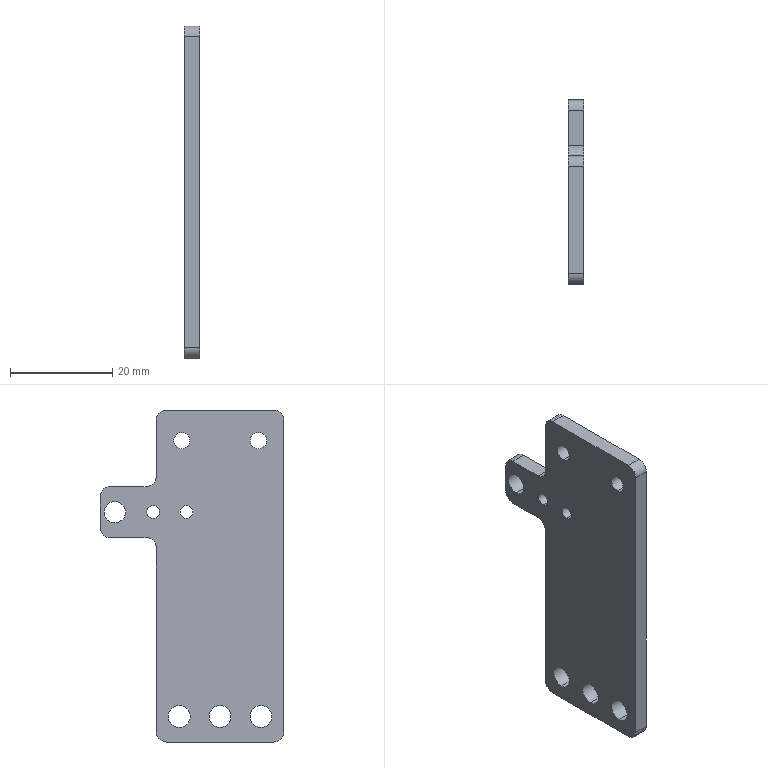Part | SolidWorks | features Fillet 2, HoleWzd 2, ICE 2, Extrusion 1 | 1 solid | 34 faces | box 3 x 36 x 65 mm | volume 4945 mm3 | cylinder 24 | plane 10 | commonest cylinder face diameters 4 x8 4.3 x6 2.5 x4 3.2 x4 4.2 x2
STEP:
#1=CARTESIAN_POINT('',(3.,6.6,13.75));
#2=VERTEX_POINT('',#1);
#3=CARTESIAN_POINT('',(3.,6.6,11.25));
#4=VERTEX_POINT('',#3);
#5=CARTESIAN_POINT('',(3.,6.6,12.5));
#6=DIRECTION('',(1.,0.,0.));
#7=DIRECTION('',(0.,0.,-1.));
#8=AXIS2_PLACEMENT_3D('',#5,#6,#7);
#9=CIRCLE('',#8,1.25);
#10=EDGE_CURVE('',#2,#4,#9,.T.);
#11=ORIENTED_EDGE('',*,*,#10,.T.);
#12=CARTESIAN_POINT('',(0.,6.6,11.25));
#13=VERTEX_POINT('',#12);
#14=CARTESIAN_POINT('',(0.,6.6,11.25));
#15=DIRECTION('',(-1.,0.,0.));
#16=VECTOR('',#15,1000.);
#17=LINE('',#14,#16);
#18=EDGE_CURVE('',#4,#13,#17,.T.);
#19=ORIENTED_EDGE('',*,*,#18,.T.);
#20=CARTESIAN_POINT('',(0.,6.6,13.75));
#21=VERTEX_POINT('',#20);
#22=CARTESIAN_POINT('',(0.,6.6,12.5));
#23=DIRECTION('',(-1.,0.,0.));
#24=DIRECTION('',(0.,0.,1.));
#25=AXIS2_PLACEMENT_3D('',#22,#23,#24);
#26=CIRCLE('',#25,1.25);
#27=EDGE_CURVE('',#13,#21,#26,.T.);
#28=ORIENTED_EDGE('',*,*,#27,.T.);
#29=CARTESIAN_POINT('',(0.,6.6,13.75));
#30=DIRECTION('',(-1.,0.,0.));
#31=VECTOR('',#30,1000.);
#32=LINE('',#29,#31);
#33=EDGE_CURVE('',#2,#21,#32,.T.);
#34=ORIENTED_EDGE('',*,*,#33,.F.);
#35=EDGE_LOOP('',(#11,#19,#28,#34));
#36=FACE_OUTER_BOUND('',#35,.T.);
#37=CARTESIAN_POINT('',(0.,6.6,12.5));
#38=DIRECTION('',(-1.,0.,0.));
#39=DIRECTION('',(0.,0.,1.));
#40=AXIS2_PLACEMENT_3D('',#37,#38,#39);
#41=CYLINDRICAL_SURFACE('',#40,1.25);
#42=ADVANCED_FACE('',(#36),#41,.F.);
#43=CARTESIAN_POINT('',(3.,13.1,13.75));
#44=VERTEX_POINT('',#43);
#45=CARTESIAN_POINT('',(3.,13.1,11.25));
#46=VERTEX_POINT('',#45);
#47=CARTESIAN_POINT('',(3.,13.1,12.5));
#48=DIRECTION('',(1.,0.,0.));
#49=DIRECTION('',(0.,0.,-1.));
#50=AXIS2_PLACEMENT_3D('',#47,#48,#49);
#51=CIRCLE('',#50,1.25);
#52=EDGE_CURVE('',#44,#46,#51,.T.);
#53=ORIENTED_EDGE('',*,*,#52,.T.);
#54=CARTESIAN_POINT('',(0.,13.1,11.25));
#55=VERTEX_POINT('',#54);
#56=CARTESIAN_POINT('',(0.,13.1,11.25));
#57=DIRECTION('',(-1.,0.,0.));
#58=VECTOR('',#57,1000.);
#59=LINE('',#56,#58);
#60=EDGE_CURVE('',#46,#55,#59,.T.);
#61=ORIENTED_EDGE('',*,*,#60,.T.);
#62=CARTESIAN_POINT('',(0.,13.1,13.75));
#63=VERTEX_POINT('',#62);
#64=CARTESIAN_POINT('',(0.,13.1,12.5));
#65=DIRECTION('',(-1.,0.,0.));
#66=DIRECTION('',(0.,0.,1.));
#67=AXIS2_PLACEMENT_3D('',#64,#65,#66);
#68=CIRCLE('',#67,1.25);
#69=EDGE_CURVE('',#55,#63,#68,.T.);
#70=ORIENTED_EDGE('',*,*,#69,.T.);
#71=CARTESIAN_POINT('',(0.,13.1,13.75));
#72=DIRECTION('',(-1.,0.,0.));
#73=VECTOR('',#72,1000.);
#74=LINE('',#71,#73);
#75=EDGE_CURVE('',#44,#63,#74,.T.);
#76=ORIENTED_EDGE('',*,*,#75,.F.);
#77=EDGE_LOOP('',(#53,#61,#70,#76));
#78=FACE_OUTER_BOUND('',#77,.T.);
#79=CARTESIAN_POINT('',(0.,13.1,12.5));
#80=DIRECTION('',(-1.,0.,0.));
#81=DIRECTION('',(0.,0.,1.));
#82=AXIS2_PLACEMENT_3D('',#79,#80,#81);
#83=CYLINDRICAL_SURFACE('',#82,1.25);
#84=ADVANCED_FACE('',(#78),#83,.F.);
#85=CARTESIAN_POINT('',(3.,20.6,14.6));
#86=VERTEX_POINT('',#85);
#87=CARTESIAN_POINT('',(3.,20.6,10.4));
#88=VERTEX_POINT('',#87);
#89=CARTESIAN_POINT('',(3.,20.6,12.5));
#90=DIRECTION('',(1.,0.,0.));
#91=DIRECTION('',(0.,0.,-1.));
#92=AXIS2_PLACEMENT_3D('',#89,#90,#91);
#93=CIRCLE('',#92,2.1);
#94=EDGE_CURVE('',#86,#88,#93,.T.);
#95=ORIENTED_EDGE('',*,*,#94,.T.);
#96=CARTESIAN_POINT('',(0.,20.6,10.4));
#97=VERTEX_POINT('',#96);
#98=CARTESIAN_POINT('',(10.,20.6,10.4));
#99=DIRECTION('',(-1.,0.,0.));
#100=VECTOR('',#99,1000.);
#101=LINE('',#98,#100);
#102=EDGE_CURVE('',#88,#97,#101,.T.);
#103=ORIENTED_EDGE('',*,*,#102,.T.);
#104=CARTESIAN_POINT('',(0.,20.6,14.6));
#105=VERTEX_POINT('',#104);
#106=CARTESIAN_POINT('',(0.,20.6,12.5));
#107=DIRECTION('',(-1.,0.,0.));
#108=DIRECTION('',(0.,0.,1.));
#109=AXIS2_PLACEMENT_3D('',#106,#107,#108);
#110=CIRCLE('',#109,2.1);
#111=EDGE_CURVE('',#97,#105,#110,.T.);
#112=ORIENTED_EDGE('',*,*,#111,.T.);
#113=CARTESIAN_POINT('',(10.,20.6,14.6));
#114=DIRECTION('',(-1.,0.,0.));
#115=VECTOR('',#114,1000.);
#116=LINE('',#113,#115);
#117=EDGE_CURVE('',#86,#105,#116,.T.);
#118=ORIENTED_EDGE('',*,*,#117,.F.);
#119=EDGE_LOOP('',(#95,#103,#112,#118));
#120=FACE_OUTER_BOUND('',#119,.T.);
#121=CARTESIAN_POINT('',(10.,20.6,12.5));
#122=DIRECTION('',(-1.,0.,0.));
#123=DIRECTION('',(0.,0.,1.));
#124=AXIS2_PLACEMENT_3D('',#121,#122,#123);
#125=CYLINDRICAL_SURFACE('',#124,2.1);
#126=ADVANCED_FACE('',(#120),#125,.F.);
#127=CARTESIAN_POINT('',(3.,8.,-25.35));
#128=VERTEX_POINT('',#127);
#129=CARTESIAN_POINT('',(3.,8.,-29.65));
#130=VERTEX_POINT('',#129);
#131=CARTESIAN_POINT('',(3.,8.,-27.5));
#132=DIRECTION('',(1.,0.,0.));
#133=DIRECTION('',(0.,0.,-1.));
#134=AXIS2_PLACEMENT_3D('',#131,#132,#133);
#135=CIRCLE('',#134,2.15);
#136=EDGE_CURVE('',#128,#130,#135,.T.);
#137=ORIENTED_EDGE('',*,*,#136,.T.);
#138=CARTESIAN_POINT('',(0.,8.,-29.65));
#139=VERTEX_POINT('',#138);
#140=CARTESIAN_POINT('',(0.,8.,-29.65));
#141=DIRECTION('',(-1.,0.,0.));
#142=VECTOR('',#141,1000.);
#143=LINE('',#140,#142);
#144=EDGE_CURVE('',#130,#139,#143,.T.);
#145=ORIENTED_EDGE('',*,*,#144,.T.);
#146=CARTESIAN_POINT('',(0.,8.,-25.35));
#147=VERTEX_POINT('',#146);
#148=CARTESIAN_POINT('',(0.,8.,-27.5));
#149=DIRECTION('',(-1.,0.,0.));
#150=DIRECTION('',(0.,0.,1.));
#151=AXIS2_PLACEMENT_3D('',#148,#149,#150);
#152=CIRCLE('',#151,2.15);
#153=EDGE_CURVE('',#139,#147,#152,.T.);
#154=ORIENTED_EDGE('',*,*,#153,.T.);
#155=CARTESIAN_POINT('',(0.,8.,-25.35));
#156=DIRECTION('',(-1.,0.,0.));
#157=VECTOR('',#156,1000.);
#158=LINE('',#155,#157);
#159=EDGE_CURVE('',#128,#147,#158,.T.);
#160=ORIENTED_EDGE('',*,*,#159,.F.);
#161=EDGE_LOOP('',(#137,#145,#154,#160));
#162=FACE_OUTER_BOUND('',#161,.T.);
#163=CARTESIAN_POINT('',(0.,8.,-27.5));
#164=DIRECTION('',(-1.,0.,0.));
#165=DIRECTION('',(0.,0.,1.));
#166=AXIS2_PLACEMENT_3D('',#163,#164,#165);
#167=CYLINDRICAL_SURFACE('',#166,2.15);
#168=ADVANCED_FACE('',(#162),#167,.F.);
#169=CARTESIAN_POINT('',(3.,-8.,-25.35));
#170=VERTEX_POINT('',#169);
#171=CARTESIAN_POINT('',(3.,-8.,-29.65));
#172=VERTEX_POINT('',#171);
#173=CARTESIAN_POINT('',(3.,-8.,-27.5));
#174=DIRECTION('',(1.,0.,0.));
#175=DIRECTION('',(0.,0.,-1.));
#176=AXIS2_PLACEMENT_3D('',#173,#174,#175);
#177=CIRCLE('',#176,2.15);
#178=EDGE_CURVE('',#170,#172,#177,.T.);
#179=ORIENTED_EDGE('',*,*,#178,.T.);
#180=CARTESIAN_POINT('',(0.,-8.,-29.65));
#181=VERTEX_POINT('',#180);
#182=CARTESIAN_POINT('',(0.,-8.,-29.65));
#183=DIRECTION('',(-1.,0.,0.));
#184=VECTOR('',#183,1000.);
#185=LINE('',#182,#184);
#186=EDGE_CURVE('',#172,#181,#185,.T.);
#187=ORIENTED_EDGE('',*,*,#186,.T.);
#188=CARTESIAN_POINT('',(0.,-8.,-25.35));
#189=VERTEX_POINT('',#188);
#190=CARTESIAN_POINT('',(0.,-8.,-27.5));
#191=DIRECTION('',(-1.,0.,0.));
#192=DIRECTION('',(0.,0.,1.));
#193=AXIS2_PLACEMENT_3D('',#190,#191,#192);
#194=CIRCLE('',#193,2.15);
#195=EDGE_CURVE('',#181,#189,#194,.T.);
#196=ORIENTED_EDGE('',*,*,#195,.T.);
#197=CARTESIAN_POINT('',(0.,-8.,-25.35));
#198=DIRECTION('',(-1.,0.,0.));
#199=VECTOR('',#198,1000.);
#200=LINE('',#197,#199);
#201=EDGE_CURVE('',#170,#189,#200,.T.);
#202=ORIENTED_EDGE('',*,*,#201,.F.);
#203=EDGE_LOOP('',(#179,#187,#196,#202));
#204=FACE_OUTER_BOUND('',#203,.T.);
#205=CARTESIAN_POINT('',(0.,-8.,-27.5));
#206=DIRECTION('',(-1.,0.,0.));
#207=DIRECTION('',(0.,0.,1.));
#208=AXIS2_PLACEMENT_3D('',#205,#206,#207);
#209=CYLINDRICAL_SURFACE('',#208,2.15);
#210=ADVANCED_FACE('',(#204),#209,.F.);
#211=CARTESIAN_POINT('',(3.,0.,-25.35));
#212=VERTEX_POINT('',#211);
#213=CARTESIAN_POINT('',(3.,0.,-29.65));
#214=VERTEX_POINT('',#213);
#215=CARTESIAN_POINT('',(3.,0.,-27.5));
#216=DIRECTION('',(1.,0.,0.));
#217=DIRECTION('',(0.,0.,-1.));
#218=AXIS2_PLACEMENT_3D('',#215,#216,#217);
#219=CIRCLE('',#218,2.15);
#220=EDGE_CURVE('',#212,#214,#219,.T.);
#221=ORIENTED_EDGE('',*,*,#220,.T.);
#222=CARTESIAN_POINT('',(0.,0.,-29.65));
#223=VERTEX_POINT('',#222);
#224=CARTESIAN_POINT('',(0.,0.,-29.65));
#225=DIRECTION('',(-1.,0.,0.));
#226=VECTOR('',#225,1000.);
#227=LINE('',#224,#226);
#228=EDGE_CURVE('',#214,#223,#227,.T.);
#229=ORIENTED_EDGE('',*,*,#228,.T.);
#230=CARTESIAN_POINT('',(0.,0.,-25.35));
#231=VERTEX_POINT('',#230);
#232=CARTESIAN_POINT('',(0.,0.,-27.5));
#233=DIRECTION('',(-1.,0.,0.));
#234=DIRECTION('',(0.,0.,1.));
#235=AXIS2_PLACEMENT_3D('',#232,#233,#234);
#236=CIRCLE('',#235,2.15);
#237=EDGE_CURVE('',#223,#231,#236,.T.);
#238=ORIENTED_EDGE('',*,*,#237,.T.);
#239=CARTESIAN_POINT('',(0.,0.,-25.35));
#240=DIRECTION('',(-1.,0.,0.));
#241=VECTOR('',#240,1000.);
#242=LINE('',#239,#241);
#243=EDGE_CURVE('',#212,#231,#242,.T.);
#244=ORIENTED_EDGE('',*,*,#243,.F.);
#245=EDGE_LOOP('',(#221,#229,#238,#244));
#246=FACE_OUTER_BOUND('',#245,.T.);
#247=CARTESIAN_POINT('',(0.,0.,-27.5));
#248=DIRECTION('',(-1.,0.,0.));
#249=DIRECTION('',(0.,0.,1.));
#250=AXIS2_PLACEMENT_3D('',#247,#248,#249);
#251=CYLINDRICAL_SURFACE('',#250,2.15);
#252=ADVANCED_FACE('',(#246),#251,.F.);
#253=CARTESIAN_POINT('',(3.,-7.5,28.1));
#254=VERTEX_POINT('',#253);
#255=CARTESIAN_POINT('',(3.,-7.5,24.9));
#256=VERTEX_POINT('',#255);
#257=CARTESIAN_POINT('',(3.,-7.5,26.5));
#258=DIRECTION('',(1.,0.,0.));
#259=DIRECTION('',(0.,0.,1.));
#260=AXIS2_PLACEMENT_3D('',#257,#258,#259);
#261=CIRCLE('',#260,1.6);
#262=EDGE_CURVE('',#254,#256,#261,.T.);
#263=ORIENTED_EDGE('',*,*,#262,.T.);
#264=CARTESIAN_POINT('',(0.,-7.5,24.9));
#265=VERTEX_POINT('',#264);
#266=CARTESIAN_POINT('',(3.,-7.5,24.9));
#267=DIRECTION('',(-1.,0.,0.));
#268=VECTOR('',#267,1000.);
#269=LINE('',#266,#268);
#270=EDGE_CURVE('',#256,#265,#269,.T.);
#271=ORIENTED_EDGE('',*,*,#270,.T.);
#272=CARTESIAN_POINT('',(0.,-7.5,28.1));
#273=VERTEX_POINT('',#272);
#274=CARTESIAN_POINT('',(0.,-7.5,26.5));
#275=DIRECTION('',(1.,0.,0.));
#276=DIRECTION('',(0.,0.,1.));
#277=AXIS2_PLACEMENT_3D('',#274,#275,#276);
#278=CIRCLE('',#277,1.6);
#279=EDGE_CURVE('',#273,#265,#278,.T.);
#280=ORIENTED_EDGE('',*,*,#279,.F.);
#281=CARTESIAN_POINT('',(3.,-7.5,28.1));
#282=DIRECTION('',(-1.,0.,0.));
#283=VECTOR('',#282,1000.);
#284=LINE('',#281,#283);
#285=EDGE_CURVE('',#254,#273,#284,.T.);
#286=ORIENTED_EDGE('',*,*,#285,.F.);
#287=EDGE_LOOP('',(#263,#271,#280,#286));
#288=FACE_OUTER_BOUND('',#287,.T.);
#289=CARTESIAN_POINT('',(3.,-7.5,26.5));
#290=DIRECTION('',(-1.,0.,0.));
#291=DIRECTION('',(0.,0.,1.));
#292=AXIS2_PLACEMENT_3D('',#289,#290,#291);
#293=CYLINDRICAL_SURFACE('',#292,1.6);
#294=ADVANCED_FACE('',(#288),#293,.F.);
#295=CARTESIAN_POINT('',(3.,7.5,28.1));
#296=VERTEX_POINT('',#295);
#297=CARTESIAN_POINT('',(3.,7.5,24.9));
#298=VERTEX_POINT('',#297);
#299=CARTESIAN_POINT('',(3.,7.5,26.5));
#300=DIRECTION('',(1.,0.,0.));
#301=DIRECTION('',(0.,0.,-1.));
#302=AXIS2_PLACEMENT_3D('',#299,#300,#301);
#303=CIRCLE('',#302,1.6);
#304=EDGE_CURVE('',#296,#298,#303,.T.);
#305=ORIENTED_EDGE('',*,*,#304,.T.);
#306=CARTESIAN_POINT('',(0.,7.5,24.9));
#307=VERTEX_POINT('',#306);
#308=CARTESIAN_POINT('',(3.,7.5,24.9));
#309=DIRECTION('',(-1.,0.,0.));
#310=VECTOR('',#309,1000.);
#311=LINE('',#308,#310);
#312=EDGE_CURVE('',#298,#307,#311,.T.);
#313=ORIENTED_EDGE('',*,*,#312,.T.);
#314=CARTESIAN_POINT('',(0.,7.5,28.1));
#315=VERTEX_POINT('',#314);
#316=CARTESIAN_POINT('',(0.,7.5,26.5));
#317=DIRECTION('',(1.,0.,0.));
#318=DIRECTION('',(0.,0.,-1.));
#319=AXIS2_PLACEMENT_3D('',#316,#317,#318);
#320=CIRCLE('',#319,1.6);
#321=EDGE_CURVE('',#315,#307,#320,.T.);
#322=ORIENTED_EDGE('',*,*,#321,.F.);
#323=CARTESIAN_POINT('',(3.,7.5,28.1));
#324=DIRECTION('',(-1.,0.,0.));
#325=VECTOR('',#324,1000.);
#326=LINE('',#323,#325);
#327=EDGE_CURVE('',#296,#315,#326,.T.);
#328=ORIENTED_EDGE('',*,*,#327,.F.);
#329=EDGE_LOOP('',(#305,#313,#322,#328));
#330=FACE_OUTER_BOUND('',#329,.T.);
#331=CARTESIAN_POINT('',(3.,7.5,26.5));
#332=DIRECTION('',(-1.,0.,0.));
#333=DIRECTION('',(0.,0.,1.));
#334=AXIS2_PLACEMENT_3D('',#331,#332,#333);
#335=CYLINDRICAL_SURFACE('',#334,1.6);
#336=ADVANCED_FACE('',(#330),#335,.F.);
#337=CARTESIAN_POINT('',(0.,12.5,-30.5));
#338=VERTEX_POINT('',#337);
#339=CARTESIAN_POINT('',(0.,12.5,5.5));
#340=VERTEX_POINT('',#339);
#341=CARTESIAN_POINT('',(0.,12.5,32.5));
#342=DIRECTION('',(0.,0.,1.));
#343=VECTOR('',#342,1000.);
#344=LINE('',#341,#343);
#345=EDGE_CURVE('',#338,#340,#344,.T.);
#346=ORIENTED_EDGE('',*,*,#345,.T.);
#347=CARTESIAN_POINT('',(3.,12.5,5.5));
#348=VERTEX_POINT('',#347);
#349=CARTESIAN_POINT('',(3.,12.5,5.5));
#350=DIRECTION('',(1.,0.,0.));
#351=VECTOR('',#350,1000.);
#352=LINE('',#349,#351);
#353=EDGE_CURVE('',#340,#348,#352,.T.);
#354=ORIENTED_EDGE('',*,*,#353,.T.);
#355=CARTESIAN_POINT('',(3.,12.5,-30.5));
#356=VERTEX_POINT('',#355);
#357=CARTESIAN_POINT('',(3.,12.5,32.5));
#358=DIRECTION('',(0.,0.,1.));
#359=VECTOR('',#358,1000.);
#360=LINE('',#357,#359);
#361=EDGE_CURVE('',#356,#348,#360,.T.);
#362=ORIENTED_EDGE('',*,*,#361,.F.);
#363=CARTESIAN_POINT('',(3.,12.5,-30.5));
#364=DIRECTION('',(-1.,0.,0.));
#365=VECTOR('',#364,1000.);
#366=LINE('',#363,#365);
#367=EDGE_CURVE('',#356,#338,#366,.T.);
#368=ORIENTED_EDGE('',*,*,#367,.T.);
#369=EDGE_LOOP('',(#346,#354,#362,#368));
#370=FACE_OUTER_BOUND('',#369,.T.);
#371=CARTESIAN_POINT('',(3.,12.5,32.5));
#372=DIRECTION('',(0.,-1.,0.));
#373=DIRECTION('',(0.,0.,-1.));
#374=AXIS2_PLACEMENT_3D('',#371,#372,#373);
#375=PLANE('',#374);
#376=ADVANCED_FACE('',(#370),#375,.F.);
#377=ORIENTED_EDGE('',*,*,#10,.F.);
#378=CARTESIAN_POINT('',(3.,6.6,12.5));
#379=DIRECTION('',(1.,0.,0.));
#380=DIRECTION('',(0.,0.,-1.));
#381=AXIS2_PLACEMENT_3D('',#378,#379,#380);
#382=CIRCLE('',#381,1.25);
#383=EDGE_CURVE('',#4,#2,#382,.T.);
#384=ORIENTED_EDGE('',*,*,#383,.F.);
#385=EDGE_LOOP('',(#377,#384));
#386=FACE_BOUND('',#385,.T.);
#387=ORIENTED_EDGE('',*,*,#52,.F.);
#388=CARTESIAN_POINT('',(3.,13.1,12.5));
#389=DIRECTION('',(1.,0.,0.));
#390=DIRECTION('',(0.,0.,-1.));
#391=AXIS2_PLACEMENT_3D('',#388,#389,#390);
#392=CIRCLE('',#391,1.25);
#393=EDGE_CURVE('',#46,#44,#392,.T.);
#394=ORIENTED_EDGE('',*,*,#393,.F.);
#395=EDGE_LOOP('',(#387,#394));
#396=FACE_BOUND('',#395,.T.);
#397=ORIENTED_EDGE('',*,*,#94,.F.);
#398=CARTESIAN_POINT('',(3.,20.6,12.5));
#399=DIRECTION('',(1.,0.,0.));
#400=DIRECTION('',(0.,0.,-1.));
#401=AXIS2_PLACEMENT_3D('',#398,#399,#400);
#402=CIRCLE('',#401,2.1);
#403=EDGE_CURVE('',#88,#86,#402,.T.);
#404=ORIENTED_EDGE('',*,*,#403,.F.);
#405=EDGE_LOOP('',(#397,#404));
#406=FACE_BOUND('',#405,.T.);
#407=CARTESIAN_POINT('',(3.,23.5,9.5));
#408=VERTEX_POINT('',#407);
#409=CARTESIAN_POINT('',(3.,23.5,15.5));
#410=VERTEX_POINT('',#409);
#411=CARTESIAN_POINT('',(3.,23.5,17.5));
#412=DIRECTION('',(0.,0.,1.));
#413=VECTOR('',#412,1000.);
#414=LINE('',#411,#413);
#415=EDGE_CURVE('',#408,#410,#414,.T.);
#416=ORIENTED_EDGE('',*,*,#415,.T.);
#417=CARTESIAN_POINT('',(3.,21.5,17.5));
#418=VERTEX_POINT('',#417);
#419=CARTESIAN_POINT('',(3.,21.5,15.5));
#420=DIRECTION('',(1.,0.,0.));
#421=DIRECTION('',(0.,0.,-1.));
#422=AXIS2_PLACEMENT_3D('',#419,#420,#421);
#423=CIRCLE('',#422,2.);
#424=EDGE_CURVE('',#410,#418,#423,.T.);
#425=ORIENTED_EDGE('',*,*,#424,.T.);
#426=CARTESIAN_POINT('',(3.,14.5,17.5));
#427=VERTEX_POINT('',#426);
#428=CARTESIAN_POINT('',(3.,23.5,17.5));
#429=DIRECTION('',(0.,-1.,0.));
#430=VECTOR('',#429,1000.);
#431=LINE('',#428,#430);
#432=EDGE_CURVE('',#418,#427,#431,.T.);
#433=ORIENTED_EDGE('',*,*,#432,.T.);
#434=CARTESIAN_POINT('',(3.,12.5,19.5));
#435=VERTEX_POINT('',#434);
#436=CARTESIAN_POINT('',(3.,14.5,19.5));
#437=DIRECTION('',(-1.,0.,0.));
#438=DIRECTION('',(0.,0.,-1.));
#439=AXIS2_PLACEMENT_3D('',#436,#437,#438);
#440=CIRCLE('',#439,2.);
#441=EDGE_CURVE('',#427,#435,#440,.T.);
#442=ORIENTED_EDGE('',*,*,#441,.T.);
#443=CARTESIAN_POINT('',(3.,12.5,30.5));
#444=VERTEX_POINT('',#443);
#445=CARTESIAN_POINT('',(3.,12.5,32.5));
#446=DIRECTION('',(0.,0.,1.));
#447=VECTOR('',#446,1000.);
#448=LINE('',#445,#447);
#449=EDGE_CURVE('',#435,#444,#448,.T.);
#450=ORIENTED_EDGE('',*,*,#449,.T.);
#451=CARTESIAN_POINT('',(3.,10.5,32.5));
#452=VERTEX_POINT('',#451);
#453=CARTESIAN_POINT('',(3.,10.5,30.5));
#454=DIRECTION('',(1.,0.,0.));
#455=DIRECTION('',(0.,0.,-1.));
#456=AXIS2_PLACEMENT_3D('',#453,#454,#455);
#457=CIRCLE('',#456,2.);
#458=EDGE_CURVE('',#444,#452,#457,.T.);
#459=ORIENTED_EDGE('',*,*,#458,.T.);
#460=CARTESIAN_POINT('',(3.,-10.5,32.5));
#461=VERTEX_POINT('',#460);
#462=CARTESIAN_POINT('',(3.,12.5,32.5));
#463=DIRECTION('',(0.,-1.,0.));
#464=VECTOR('',#463,1000.);
#465=LINE('',#462,#464);
#466=EDGE_CURVE('',#452,#461,#465,.T.);
#467=ORIENTED_EDGE('',*,*,#466,.T.);
#468=CARTESIAN_POINT('',(3.,-12.5,30.5));
#469=VERTEX_POINT('',#468);
#470=CARTESIAN_POINT('',(3.,-10.5,30.5));
#471=DIRECTION('',(1.,0.,0.));
#472=DIRECTION('',(0.,0.,-1.));
#473=AXIS2_PLACEMENT_3D('',#470,#471,#472);
#474=CIRCLE('',#473,2.);
#475=EDGE_CURVE('',#461,#469,#474,.T.);
#476=ORIENTED_EDGE('',*,*,#475,.T.);
#477=CARTESIAN_POINT('',(3.,-12.5,-30.5));
#478=VERTEX_POINT('',#477);
#479=CARTESIAN_POINT('',(3.,-12.5,32.5));
#480=DIRECTION('',(0.,0.,-1.));
#481=VECTOR('',#480,1000.);
#482=LINE('',#479,#481);
#483=EDGE_CURVE('',#469,#478,#482,.T.);
#484=ORIENTED_EDGE('',*,*,#483,.T.);
#485=CARTESIAN_POINT('',(3.,-10.5,-32.5));
#486=VERTEX_POINT('',#485);
#487=CARTESIAN_POINT('',(3.,-10.5,-30.5));
#488=DIRECTION('',(1.,0.,0.));
#489=DIRECTION('',(0.,0.,-1.));
#490=AXIS2_PLACEMENT_3D('',#487,#488,#489);
#491=CIRCLE('',#490,2.);
#492=EDGE_CURVE('',#478,#486,#491,.T.);
#493=ORIENTED_EDGE('',*,*,#492,.T.);
#494=CARTESIAN_POINT('',(3.,10.5,-32.5));
#495=VERTEX_POINT('',#494);
#496=CARTESIAN_POINT('',(3.,12.5,-32.5));
#497=DIRECTION('',(0.,1.,0.));
#498=VECTOR('',#497,1000.);
#499=LINE('',#496,#498);
#500=EDGE_CURVE('',#486,#495,#499,.T.);
#501=ORIENTED_EDGE('',*,*,#500,.T.);
#502=CARTESIAN_POINT('',(3.,10.5,-30.5));
#503=DIRECTION('',(1.,0.,0.));
#504=DIRECTION('',(0.,0.,-1.));
#505=AXIS2_PLACEMENT_3D('',#502,#503,#504);
#506=CIRCLE('',#505,2.);
#507=EDGE_CURVE('',#495,#356,#506,.T.);
#508=ORIENTED_EDGE('',*,*,#507,.T.);
#509=ORIENTED_EDGE('',*,*,#361,.T.);
#510=CARTESIAN_POINT('',(3.,14.5,7.5));
#511=VERTEX_POINT('',#510);
#512=CARTESIAN_POINT('',(3.,14.5,5.5));
#513=DIRECTION('',(-1.,0.,0.));
#514=DIRECTION('',(0.,0.,-1.));
#515=AXIS2_PLACEMENT_3D('',#512,#513,#514);
#516=CIRCLE('',#515,2.);
#517=EDGE_CURVE('',#348,#511,#516,.T.);
#518=ORIENTED_EDGE('',*,*,#517,.T.);
#519=CARTESIAN_POINT('',(3.,21.5,7.5));
#520=VERTEX_POINT('',#519);
#521=CARTESIAN_POINT('',(3.,23.5,7.5));
#522=DIRECTION('',(0.,1.,0.));
#523=VECTOR('',#522,1000.);
#524=LINE('',#521,#523);
#525=EDGE_CURVE('',#511,#520,#524,.T.);
#526=ORIENTED_EDGE('',*,*,#525,.T.);
#527=CARTESIAN_POINT('',(3.,21.5,9.5));
#528=DIRECTION('',(1.,0.,0.));
#529=DIRECTION('',(0.,0.,-1.));
#530=AXIS2_PLACEMENT_3D('',#527,#528,#529);
#531=CIRCLE('',#530,2.);
#532=EDGE_CURVE('',#520,#408,#531,.T.);
#533=ORIENTED_EDGE('',*,*,#532,.T.);
#534=EDGE_LOOP('',(#416,#425,#433,#442,#450,#459,#467,#476,#484,#493,#501,#508,#509,#518,#526,#533));
#535=FACE_OUTER_BOUND('',#534,.T.);
#536=ORIENTED_EDGE('',*,*,#136,.F.);
#537=CARTESIAN_POINT('',(3.,8.,-27.5));
#538=DIRECTION('',(1.,0.,0.));
#539=DIRECTION('',(0.,0.,-1.));
#540=AXIS2_PLACEMENT_3D('',#537,#538,#539);
#541=CIRCLE('',#540,2.15);
#542=EDGE_CURVE('',#130,#128,#541,.T.);
#543=ORIENTED_EDGE('',*,*,#542,.F.);
#544=EDGE_LOOP('',(#536,#543));
#545=FACE_BOUND('',#544,.T.);
#546=ORIENTED_EDGE('',*,*,#178,.F.);
#547=CARTESIAN_POINT('',(3.,-8.,-27.5));
#548=DIRECTION('',(1.,0.,0.));
#549=DIRECTION('',(0.,0.,-1.));
#550=AXIS2_PLACEMENT_3D('',#547,#548,#549);
#551=CIRCLE('',#550,2.15);
#552=EDGE_CURVE('',#172,#170,#551,.T.);
#553=ORIENTED_EDGE('',*,*,#552,.F.);
#554=EDGE_LOOP('',(#546,#553));
#555=FACE_BOUND('',#554,.T.);
#556=ORIENTED_EDGE('',*,*,#220,.F.);
#557=CARTESIAN_POINT('',(3.,0.,-27.5));
#558=DIRECTION('',(1.,0.,0.));
#559=DIRECTION('',(0.,0.,-1.));
#560=AXIS2_PLACEMENT_3D('',#557,#558,#559);
#561=CIRCLE('',#560,2.15);
#562=EDGE_CURVE('',#214,#212,#561,.T.);
#563=ORIENTED_EDGE('',*,*,#562,.F.);
#564=EDGE_LOOP('',(#556,#563));
#565=FACE_BOUND('',#564,.T.);
#566=ORIENTED_EDGE('',*,*,#304,.F.);
#567=CARTESIAN_POINT('',(3.,7.5,26.5));
#568=DIRECTION('',(1.,0.,0.));
#569=DIRECTION('',(0.,0.,-1.));
#570=AXIS2_PLACEMENT_3D('',#567,#568,#569);
#571=CIRCLE('',#570,1.6);
#572=EDGE_CURVE('',#298,#296,#571,.T.);
#573=ORIENTED_EDGE('',*,*,#572,.F.);
#574=EDGE_LOOP('',(#566,#573));
#575=FACE_BOUND('',#574,.T.);
#576=ORIENTED_EDGE('',*,*,#262,.F.);
#577=CARTESIAN_POINT('',(3.,-7.5,26.5));
#578=DIRECTION('',(1.,0.,0.));
#579=DIRECTION('',(0.,0.,1.));
#580=AXIS2_PLACEMENT_3D('',#577,#578,#579);
#581=CIRCLE('',#580,1.6);
#582=EDGE_CURVE('',#256,#254,#581,.T.);
#583=ORIENTED_EDGE('',*,*,#582,.F.);
#584=EDGE_LOOP('',(#576,#583));
#585=FACE_BOUND('',#584,.T.);
#586=CARTESIAN_POINT('',(3.,0.,0.));
#587=DIRECTION('',(1.,0.,0.));
#588=DIRECTION('',(0.,0.,-1.));
#589=AXIS2_PLACEMENT_3D('',#586,#587,#588);
#590=PLANE('',#589);
#591=ADVANCED_FACE('',(#386,#396,#406,#535,#545,#555,#565,#575,#585),#590,.T.);
#592=CARTESIAN_POINT('',(0.,6.6,12.5));
#593=DIRECTION('',(-1.,0.,0.));
#594=DIRECTION('',(0.,0.,1.));
#595=AXIS2_PLACEMENT_3D('',#592,#593,#594);
#596=CIRCLE('',#595,1.25);
#597=EDGE_CURVE('',#21,#13,#596,.T.);
#598=ORIENTED_EDGE('',*,*,#597,.F.);
#599=ORIENTED_EDGE('',*,*,#27,.F.);
#600=EDGE_LOOP('',(#598,#599));
#601=FACE_BOUND('',#600,.T.);
#602=CARTESIAN_POINT('',(0.,13.1,12.5));
#603=DIRECTION('',(-1.,0.,0.));
#604=DIRECTION('',(0.,0.,1.));
#605=AXIS2_PLACEMENT_3D('',#602,#603,#604);
#606=CIRCLE('',#605,1.25);
#607=EDGE_CURVE('',#63,#55,#606,.T.);
#608=ORIENTED_EDGE('',*,*,#607,.F.);
#609=ORIENTED_EDGE('',*,*,#69,.F.);
#610=EDGE_LOOP('',(#608,#609));
#611=FACE_BOUND('',#610,.T.);
#612=CARTESIAN_POINT('',(0.,20.6,12.5));
#613=DIRECTION('',(-1.,0.,0.));
#614=DIRECTION('',(0.,0.,1.));
#615=AXIS2_PLACEMENT_3D('',#612,#613,#614);
#616=CIRCLE('',#615,2.1);
#617=EDGE_CURVE('',#105,#97,#616,.T.);
#618=ORIENTED_EDGE('',*,*,#617,.F.);
#619=ORIENTED_EDGE('',*,*,#111,.F.);
#620=EDGE_LOOP('',(#618,#619));
#621=FACE_BOUND('',#620,.T.);
#622=CARTESIAN_POINT('',(0.,14.5,17.5));
#623=VERTEX_POINT('',#622);
#624=CARTESIAN_POINT('',(0.,21.5,17.5));
#625=VERTEX_POINT('',#624);
#626=CARTESIAN_POINT('',(0.,23.5,17.5));
#627=DIRECTION('',(0.,1.,0.));
#628=VECTOR('',#627,1000.);
#629=LINE('',#626,#628);
#630=EDGE_CURVE('',#623,#625,#629,.T.);
#631=ORIENTED_EDGE('',*,*,#630,.T.);
#632=CARTESIAN_POINT('',(0.,23.5,15.5));
#633=VERTEX_POINT('',#632);
#634=CARTESIAN_POINT('',(0.,21.5,15.5));
#635=DIRECTION('',(-1.,0.,0.));
#636=DIRECTION('',(0.,0.,-1.));
#637=AXIS2_PLACEMENT_3D('',#634,#635,#636);
#638=CIRCLE('',#637,2.);
#639=EDGE_CURVE('',#625,#633,#638,.T.);
#640=ORIENTED_EDGE('',*,*,#639,.T.);
#641=CARTESIAN_POINT('',(0.,23.5,9.5));
#642=VERTEX_POINT('',#641);
#643=CARTESIAN_POINT('',(0.,23.5,17.5));
#644=DIRECTION('',(0.,0.,-1.));
#645=VECTOR('',#644,1000.);
#646=LINE('',#643,#645);
#647=EDGE_CURVE('',#633,#642,#646,.T.);
#648=ORIENTED_EDGE('',*,*,#647,.T.);
#649=CARTESIAN_POINT('',(0.,21.5,7.5));
#650=VERTEX_POINT('',#649);
#651=CARTESIAN_POINT('',(0.,21.5,9.5));
#652=DIRECTION('',(-1.,0.,0.));
#653=DIRECTION('',(0.,0.,-1.));
#654=AXIS2_PLACEMENT_3D('',#651,#652,#653);
#655=CIRCLE('',#654,2.);
#656=EDGE_CURVE('',#642,#650,#655,.T.);
#657=ORIENTED_EDGE('',*,*,#656,.T.);
#658=CARTESIAN_POINT('',(0.,14.5,7.5));
#659=VERTEX_POINT('',#658);
#660=CARTESIAN_POINT('',(0.,23.5,7.5));
#661=DIRECTION('',(0.,-1.,0.));
#662=VECTOR('',#661,1000.);
#663=LINE('',#660,#662);
#664=EDGE_CURVE('',#650,#659,#663,.T.);
#665=ORIENTED_EDGE('',*,*,#664,.T.);
#666=CARTESIAN_POINT('',(0.,14.5,5.5));
#667=DIRECTION('',(1.,0.,0.));
#668=DIRECTION('',(0.,0.,-1.));
#669=AXIS2_PLACEMENT_3D('',#666,#667,#668);
#670=CIRCLE('',#669,2.);
#671=EDGE_CURVE('',#659,#340,#670,.T.);
#672=ORIENTED_EDGE('',*,*,#671,.T.);
#673=ORIENTED_EDGE('',*,*,#345,.F.);
#674=CARTESIAN_POINT('',(0.,10.5,-32.5));
#675=VERTEX_POINT('',#674);
#676=CARTESIAN_POINT('',(0.,10.5,-30.5));
#677=DIRECTION('',(-1.,0.,0.));
#678=DIRECTION('',(0.,0.,-1.));
#679=AXIS2_PLACEMENT_3D('',#676,#677,#678);
#680=CIRCLE('',#679,2.);
#681=EDGE_CURVE('',#338,#675,#680,.T.);
#682=ORIENTED_EDGE('',*,*,#681,.T.);
#683=CARTESIAN_POINT('',(0.,-10.5,-32.5));
#684=VERTEX_POINT('',#683);
#685=CARTESIAN_POINT('',(0.,12.5,-32.5));
#686=DIRECTION('',(0.,1.,0.));
#687=VECTOR('',#686,1000.);
#688=LINE('',#685,#687);
#689=EDGE_CURVE('',#684,#675,#688,.T.);
#690=ORIENTED_EDGE('',*,*,#689,.F.);
#691=CARTESIAN_POINT('',(0.,-12.5,-30.5));
#692=VERTEX_POINT('',#691);
#693=CARTESIAN_POINT('',(0.,-10.5,-30.5));
#694=DIRECTION('',(-1.,0.,0.));
#695=DIRECTION('',(0.,0.,-1.));
#696=AXIS2_PLACEMENT_3D('',#693,#694,#695);
#697=CIRCLE('',#696,2.);
#698=EDGE_CURVE('',#684,#692,#697,.T.);
#699=ORIENTED_EDGE('',*,*,#698,.T.);
#700=CARTESIAN_POINT('',(0.,-12.5,30.5));
#701=VERTEX_POINT('',#700);
#702=CARTESIAN_POINT('',(0.,-12.5,32.5));
#703=DIRECTION('',(0.,0.,-1.));
#704=VECTOR('',#703,1000.);
#705=LINE('',#702,#704);
#706=EDGE_CURVE('',#701,#692,#705,.T.);
#707=ORIENTED_EDGE('',*,*,#706,.F.);
#708=CARTESIAN_POINT('',(0.,-10.5,32.5));
#709=VERTEX_POINT('',#708);
#710=CARTESIAN_POINT('',(0.,-10.5,30.5));
#711=DIRECTION('',(-1.,0.,0.));
#712=DIRECTION('',(0.,0.,-1.));
#713=AXIS2_PLACEMENT_3D('',#710,#711,#712);
#714=CIRCLE('',#713,2.);
#715=EDGE_CURVE('',#701,#709,#714,.T.);
#716=ORIENTED_EDGE('',*,*,#715,.T.);
#717=CARTESIAN_POINT('',(0.,10.5,32.5));
#718=VERTEX_POINT('',#717);
#719=CARTESIAN_POINT('',(0.,12.5,32.5));
#720=DIRECTION('',(0.,-1.,0.));
#721=VECTOR('',#720,1000.);
#722=LINE('',#719,#721);
#723=EDGE_CURVE('',#718,#709,#722,.T.);
#724=ORIENTED_EDGE('',*,*,#723,.F.);
#725=CARTESIAN_POINT('',(0.,12.5,30.5));
#726=VERTEX_POINT('',#725);
#727=CARTESIAN_POINT('',(0.,10.5,30.5));
#728=DIRECTION('',(-1.,0.,0.));
#729=DIRECTION('',(0.,0.,-1.));
#730=AXIS2_PLACEMENT_3D('',#727,#728,#729);
#731=CIRCLE('',#730,2.);
#732=EDGE_CURVE('',#718,#726,#731,.T.);
#733=ORIENTED_EDGE('',*,*,#732,.T.);
#734=CARTESIAN_POINT('',(0.,12.5,19.5));
#735=VERTEX_POINT('',#734);
#736=CARTESIAN_POINT('',(0.,12.5,32.5));
#737=DIRECTION('',(0.,0.,1.));
#738=VECTOR('',#737,1000.);
#739=LINE('',#736,#738);
#740=EDGE_CURVE('',#735,#726,#739,.T.);
#741=ORIENTED_EDGE('',*,*,#740,.F.);
#742=CARTESIAN_POINT('',(0.,14.5,19.5));
#743=DIRECTION('',(1.,0.,0.));
#744=DIRECTION('',(0.,0.,-1.));
#745=AXIS2_PLACEMENT_3D('',#742,#743,#744);
#746=CIRCLE('',#745,2.);
#747=EDGE_CURVE('',#735,#623,#746,.T.);
#748=ORIENTED_EDGE('',*,*,#747,.T.);
#749=EDGE_LOOP('',(#631,#640,#648,#657,#665,#672,#673,#682,#690,#699,#707,#716,#724,#733,#741,#748));
#750=FACE_OUTER_BOUND('',#749,.T.);
#751=CARTESIAN_POINT('',(0.,8.,-27.5));
#752=DIRECTION('',(-1.,0.,0.));
#753=DIRECTION('',(0.,0.,1.));
#754=AXIS2_PLACEMENT_3D('',#751,#752,#753);
#755=CIRCLE('',#754,2.15);
#756=EDGE_CURVE('',#147,#139,#755,.T.);
#757=ORIENTED_EDGE('',*,*,#756,.F.);
#758=ORIENTED_EDGE('',*,*,#153,.F.);
#759=EDGE_LOOP('',(#757,#758));
#760=FACE_BOUND('',#759,.T.);
#761=CARTESIAN_POINT('',(0.,-8.,-27.5));
#762=DIRECTION('',(-1.,0.,0.));
#763=DIRECTION('',(0.,0.,1.));
#764=AXIS2_PLACEMENT_3D('',#761,#762,#763);
#765=CIRCLE('',#764,2.15);
#766=EDGE_CURVE('',#189,#181,#765,.T.);
#767=ORIENTED_EDGE('',*,*,#766,.F.);
#768=ORIENTED_EDGE('',*,*,#195,.F.);
#769=EDGE_LOOP('',(#767,#768));
#770=FACE_BOUND('',#769,.T.);
#771=CARTESIAN_POINT('',(0.,0.,-27.5));
#772=DIRECTION('',(-1.,0.,0.));
#773=DIRECTION('',(0.,0.,1.));
#774=AXIS2_PLACEMENT_3D('',#771,#772,#773);
#775=CIRCLE('',#774,2.15);
#776=EDGE_CURVE('',#231,#223,#775,.T.);
#777=ORIENTED_EDGE('',*,*,#776,.F.);
#778=ORIENTED_EDGE('',*,*,#237,.F.);
#779=EDGE_LOOP('',(#777,#778));
#780=FACE_BOUND('',#779,.T.);
#781=ORIENTED_EDGE('',*,*,#321,.T.);
#782=CARTESIAN_POINT('',(0.,7.5,26.5));
#783=DIRECTION('',(1.,0.,0.));
#784=DIRECTION('',(0.,0.,-1.));
#785=AXIS2_PLACEMENT_3D('',#782,#783,#784);
#786=CIRCLE('',#785,1.6);
#787=EDGE_CURVE('',#307,#315,#786,.T.);
#788=ORIENTED_EDGE('',*,*,#787,.T.);
#789=EDGE_LOOP('',(#781,#788));
#790=FACE_BOUND('',#789,.T.);
#791=ORIENTED_EDGE('',*,*,#279,.T.);
#792=CARTESIAN_POINT('',(0.,-7.5,26.5));
#793=DIRECTION('',(1.,0.,0.));
#794=DIRECTION('',(0.,0.,1.));
#795=AXIS2_PLACEMENT_3D('',#792,#793,#794);
#796=CIRCLE('',#795,1.6);
#797=EDGE_CURVE('',#265,#273,#796,.T.);
#798=ORIENTED_EDGE('',*,*,#797,.T.);
#799=EDGE_LOOP('',(#791,#798));
#800=FACE_BOUND('',#799,.T.);
#801=CARTESIAN_POINT('',(0.,0.,0.));
#802=DIRECTION('',(1.,0.,0.));
#803=DIRECTION('',(0.,0.,-1.));
#804=AXIS2_PLACEMENT_3D('',#801,#802,#803);
#805=PLANE('',#804);
#806=ADVANCED_FACE('',(#601,#611,#621,#750,#760,#770,#780,#790,#800),#805,.F.);
#807=ORIENTED_EDGE('',*,*,#500,.F.);
#808=CARTESIAN_POINT('',(3.,-10.5,-32.5));
#809=DIRECTION('',(-1.,0.,0.));
#810=VECTOR('',#809,1000.);
#811=LINE('',#808,#810);
#812=EDGE_CURVE('',#486,#684,#811,.T.);
#813=ORIENTED_EDGE('',*,*,#812,.T.);
#814=ORIENTED_EDGE('',*,*,#689,.T.);
#815=CARTESIAN_POINT('',(3.,10.5,-32.5));
#816=DIRECTION('',(1.,0.,0.));
#817=VECTOR('',#816,1000.);
#818=LINE('',#815,#817);
#819=EDGE_CURVE('',#675,#495,#818,.T.);
#820=ORIENTED_EDGE('',*,*,#819,.T.);
#821=EDGE_LOOP('',(#807,#813,#814,#820));
#822=FACE_OUTER_BOUND('',#821,.T.);
#823=CARTESIAN_POINT('',(3.,12.5,-32.5));
#824=DIRECTION('',(0.,0.,1.));
#825=DIRECTION('',(1.,0.,0.));
#826=AXIS2_PLACEMENT_3D('',#823,#824,#825);
#827=PLANE('',#826);
#828=ADVANCED_FACE('',(#822),#827,.F.);
#829=ORIENTED_EDGE('',*,*,#449,.F.);
#830=CARTESIAN_POINT('',(3.,12.5,19.5));
#831=DIRECTION('',(-1.,0.,0.));
#832=VECTOR('',#831,1000.);
#833=LINE('',#830,#832);
#834=EDGE_CURVE('',#435,#735,#833,.T.);
#835=ORIENTED_EDGE('',*,*,#834,.T.);
#836=ORIENTED_EDGE('',*,*,#740,.T.);
#837=CARTESIAN_POINT('',(3.,12.5,30.5));
#838=DIRECTION('',(1.,0.,0.));
#839=VECTOR('',#838,1000.);
#840=LINE('',#837,#839);
#841=EDGE_CURVE('',#726,#444,#840,.T.);
#842=ORIENTED_EDGE('',*,*,#841,.T.);
#843=EDGE_LOOP('',(#829,#835,#836,#842));
#844=FACE_OUTER_BOUND('',#843,.T.);
#845=CARTESIAN_POINT('',(3.,12.5,32.5));
#846=DIRECTION('',(0.,-1.,0.));
#847=DIRECTION('',(0.,0.,-1.));
#848=AXIS2_PLACEMENT_3D('',#845,#846,#847);
#849=PLANE('',#848);
#850=ADVANCED_FACE('',(#844),#849,.F.);
#851=ORIENTED_EDGE('',*,*,#723,.T.);
#852=CARTESIAN_POINT('',(3.,-10.5,32.5));
#853=DIRECTION('',(1.,0.,0.));
#854=VECTOR('',#853,1000.);
#855=LINE('',#852,#854);
#856=EDGE_CURVE('',#709,#461,#855,.T.);
#857=ORIENTED_EDGE('',*,*,#856,.T.);
#858=ORIENTED_EDGE('',*,*,#466,.F.);
#859=CARTESIAN_POINT('',(3.,10.5,32.5));
#860=DIRECTION('',(-1.,0.,0.));
#861=VECTOR('',#860,1000.);
#862=LINE('',#859,#861);
#863=EDGE_CURVE('',#452,#718,#862,.T.);
#864=ORIENTED_EDGE('',*,*,#863,.T.);
#865=EDGE_LOOP('',(#851,#857,#858,#864));
#866=FACE_OUTER_BOUND('',#865,.T.);
#867=CARTESIAN_POINT('',(3.,12.5,32.5));
#868=DIRECTION('',(0.,0.,-1.));
#869=DIRECTION('',(-1.,0.,0.));
#870=AXIS2_PLACEMENT_3D('',#867,#868,#869);
#871=PLANE('',#870);
#872=ADVANCED_FACE('',(#866),#871,.F.);
#873=ORIENTED_EDGE('',*,*,#706,.T.);
#874=CARTESIAN_POINT('',(3.,-12.5,-30.5));
#875=DIRECTION('',(1.,0.,0.));
#876=VECTOR('',#875,1000.);
#877=LINE('',#874,#876);
#878=EDGE_CURVE('',#692,#478,#877,.T.);
#879=ORIENTED_EDGE('',*,*,#878,.T.);
#880=ORIENTED_EDGE('',*,*,#483,.F.);
#881=CARTESIAN_POINT('',(3.,-12.5,30.5));
#882=DIRECTION('',(-1.,0.,0.));
#883=VECTOR('',#882,1000.);
#884=LINE('',#881,#883);
#885=EDGE_CURVE('',#469,#701,#884,.T.);
#886=ORIENTED_EDGE('',*,*,#885,.T.);
#887=EDGE_LOOP('',(#873,#879,#880,#886));
#888=FACE_OUTER_BOUND('',#887,.T.);
#889=CARTESIAN_POINT('',(3.,-12.5,32.5));
#890=DIRECTION('',(0.,1.,0.));
#891=DIRECTION('',(0.,0.,1.));
#892=AXIS2_PLACEMENT_3D('',#889,#890,#891);
#893=PLANE('',#892);
#894=ADVANCED_FACE('',(#888),#893,.F.);
#895=ORIENTED_EDGE('',*,*,#312,.F.);
#896=ORIENTED_EDGE('',*,*,#572,.T.);
#897=ORIENTED_EDGE('',*,*,#327,.T.);
#898=ORIENTED_EDGE('',*,*,#787,.F.);
#899=EDGE_LOOP('',(#895,#896,#897,#898));
#900=FACE_OUTER_BOUND('',#899,.T.);
#901=CARTESIAN_POINT('',(3.,7.5,26.5));
#902=DIRECTION('',(-1.,0.,0.));
#903=DIRECTION('',(0.,0.,1.));
#904=AXIS2_PLACEMENT_3D('',#901,#902,#903);
#905=CYLINDRICAL_SURFACE('',#904,1.6);
#906=ADVANCED_FACE('',(#900),#905,.F.);
#907=ORIENTED_EDGE('',*,*,#270,.F.);
#908=ORIENTED_EDGE('',*,*,#582,.T.);
#909=ORIENTED_EDGE('',*,*,#285,.T.);
#910=ORIENTED_EDGE('',*,*,#797,.F.);
#911=EDGE_LOOP('',(#907,#908,#909,#910));
#912=FACE_OUTER_BOUND('',#911,.T.);
#913=CARTESIAN_POINT('',(3.,-7.5,26.5));
#914=DIRECTION('',(-1.,0.,0.));
#915=DIRECTION('',(0.,0.,1.));
#916=AXIS2_PLACEMENT_3D('',#913,#914,#915);
#917=CYLINDRICAL_SURFACE('',#916,1.6);
#918=ADVANCED_FACE('',(#912),#917,.F.);
#919=ORIENTED_EDGE('',*,*,#492,.F.);
#920=ORIENTED_EDGE('',*,*,#878,.F.);
#921=ORIENTED_EDGE('',*,*,#698,.F.);
#922=ORIENTED_EDGE('',*,*,#812,.F.);
#923=EDGE_LOOP('',(#919,#920,#921,#922));
#924=FACE_OUTER_BOUND('',#923,.T.);
#925=CARTESIAN_POINT('',(3.,-10.5,-30.5));
#926=DIRECTION('',(-1.,0.,0.));
#927=DIRECTION('',(0.,0.,1.));
#928=AXIS2_PLACEMENT_3D('',#925,#926,#927);
#929=CYLINDRICAL_SURFACE('',#928,2.);
#930=ADVANCED_FACE('',(#924),#929,.T.);
#931=ORIENTED_EDGE('',*,*,#507,.F.);
#932=ORIENTED_EDGE('',*,*,#819,.F.);
#933=ORIENTED_EDGE('',*,*,#681,.F.);
#934=ORIENTED_EDGE('',*,*,#367,.F.);
#935=EDGE_LOOP('',(#931,#932,#933,#934));
#936=FACE_OUTER_BOUND('',#935,.T.);
#937=CARTESIAN_POINT('',(3.,10.5,-30.5));
#938=DIRECTION('',(-1.,0.,0.));
#939=DIRECTION('',(0.,0.,1.));
#940=AXIS2_PLACEMENT_3D('',#937,#938,#939);
#941=CYLINDRICAL_SURFACE('',#940,2.);
#942=ADVANCED_FACE('',(#936),#941,.T.);
#943=ORIENTED_EDGE('',*,*,#475,.F.);
#944=ORIENTED_EDGE('',*,*,#856,.F.);
#945=ORIENTED_EDGE('',*,*,#715,.F.);
#946=ORIENTED_EDGE('',*,*,#885,.F.);
#947=EDGE_LOOP('',(#943,#944,#945,#946));
#948=FACE_OUTER_BOUND('',#947,.T.);
#949=CARTESIAN_POINT('',(3.,-10.5,30.5));
#950=DIRECTION('',(-1.,0.,0.));
#951=DIRECTION('',(0.,0.,1.));
#952=AXIS2_PLACEMENT_3D('',#949,#950,#951);
#953=CYLINDRICAL_SURFACE('',#952,2.);
#954=ADVANCED_FACE('',(#948),#953,.T.);
#955=ORIENTED_EDGE('',*,*,#458,.F.);
#956=ORIENTED_EDGE('',*,*,#841,.F.);
#957=ORIENTED_EDGE('',*,*,#732,.F.);
#958=ORIENTED_EDGE('',*,*,#863,.F.);
#959=EDGE_LOOP('',(#955,#956,#957,#958));
#960=FACE_OUTER_BOUND('',#959,.T.);
#961=CARTESIAN_POINT('',(3.,10.5,30.5));
#962=DIRECTION('',(-1.,0.,0.));
#963=DIRECTION('',(0.,0.,1.));
#964=AXIS2_PLACEMENT_3D('',#961,#962,#963);
#965=CYLINDRICAL_SURFACE('',#964,2.);
#966=ADVANCED_FACE('',(#960),#965,.T.);
#967=ORIENTED_EDGE('',*,*,#228,.F.);
#968=ORIENTED_EDGE('',*,*,#562,.T.);
#969=ORIENTED_EDGE('',*,*,#243,.T.);
#970=ORIENTED_EDGE('',*,*,#776,.T.);
#971=EDGE_LOOP('',(#967,#968,#969,#970));
#972=FACE_OUTER_BOUND('',#971,.T.);
#973=CARTESIAN_POINT('',(0.,0.,-27.5));
#974=DIRECTION('',(-1.,0.,0.));
#975=DIRECTION('',(0.,0.,1.));
#976=AXIS2_PLACEMENT_3D('',#973,#974,#975);
#977=CYLINDRICAL_SURFACE('',#976,2.15);
#978=ADVANCED_FACE('',(#972),#977,.F.);
#979=ORIENTED_EDGE('',*,*,#186,.F.);
#980=ORIENTED_EDGE('',*,*,#552,.T.);
#981=ORIENTED_EDGE('',*,*,#201,.T.);
#982=ORIENTED_EDGE('',*,*,#766,.T.);
#983=EDGE_LOOP('',(#979,#980,#981,#982));
#984=FACE_OUTER_BOUND('',#983,.T.);
#985=CARTESIAN_POINT('',(0.,-8.,-27.5));
#986=DIRECTION('',(-1.,0.,0.));
#987=DIRECTION('',(0.,0.,1.));
#988=AXIS2_PLACEMENT_3D('',#985,#986,#987);
#989=CYLINDRICAL_SURFACE('',#988,2.15);
#990=ADVANCED_FACE('',(#984),#989,.F.);
#991=ORIENTED_EDGE('',*,*,#144,.F.);
#992=ORIENTED_EDGE('',*,*,#542,.T.);
#993=ORIENTED_EDGE('',*,*,#159,.T.);
#994=ORIENTED_EDGE('',*,*,#756,.T.);
#995=EDGE_LOOP('',(#991,#992,#993,#994));
#996=FACE_OUTER_BOUND('',#995,.T.);
#997=CARTESIAN_POINT('',(0.,8.,-27.5));
#998=DIRECTION('',(-1.,0.,0.));
#999=DIRECTION('',(0.,0.,1.));
#1000=AXIS2_PLACEMENT_3D('',#997,#998,#999);
#1001=CYLINDRICAL_SURFACE('',#1000,2.15);
#1002=ADVANCED_FACE('',(#996),#1001,.F.);
#1003=ORIENTED_EDGE('',*,*,#664,.F.);
#1004=CARTESIAN_POINT('',(-24.166,21.5,7.5));
#1005=DIRECTION('',(1.,0.,0.));
#1006=VECTOR('',#1005,1000.);
#1007=LINE('',#1004,#1006);
#1008=EDGE_CURVE('',#650,#520,#1007,.T.);
#1009=ORIENTED_EDGE('',*,*,#1008,.T.);
#1010=ORIENTED_EDGE('',*,*,#525,.F.);
#1011=CARTESIAN_POINT('',(-24.166,14.5,7.5));
#1012=DIRECTION('',(-1.,0.,0.));
#1013=VECTOR('',#1012,1000.);
#1014=LINE('',#1011,#1013);
#1015=EDGE_CURVE('',#511,#659,#1014,.T.);
#1016=ORIENTED_EDGE('',*,*,#1015,.T.);
#1017=EDGE_LOOP('',(#1003,#1009,#1010,#1016));
#1018=FACE_OUTER_BOUND('',#1017,.T.);
#1019=CARTESIAN_POINT('',(-24.166,23.5,7.5));
#1020=DIRECTION('',(0.,0.,-1.));
#1021=DIRECTION('',(0.,1.,0.));
#1022=AXIS2_PLACEMENT_3D('',#1019,#1020,#1021);
#1023=PLANE('',#1022);
#1024=ADVANCED_FACE('',(#1018),#1023,.T.);
#1025=ORIENTED_EDGE('',*,*,#432,.F.);
#1026=CARTESIAN_POINT('',(-24.166,21.5,17.5));
#1027=DIRECTION('',(-1.,0.,0.));
#1028=VECTOR('',#1027,1000.);
#1029=LINE('',#1026,#1028);
#1030=EDGE_CURVE('',#418,#625,#1029,.T.);
#1031=ORIENTED_EDGE('',*,*,#1030,.T.);
#1032=ORIENTED_EDGE('',*,*,#630,.F.);
#1033=CARTESIAN_POINT('',(-24.166,14.5,17.5));
#1034=DIRECTION('',(1.,0.,0.));
#1035=VECTOR('',#1034,1000.);
#1036=LINE('',#1033,#1035);
#1037=EDGE_CURVE('',#623,#427,#1036,.T.);
#1038=ORIENTED_EDGE('',*,*,#1037,.T.);
#1039=EDGE_LOOP('',(#1025,#1031,#1032,#1038));
#1040=FACE_OUTER_BOUND('',#1039,.T.);
#1041=CARTESIAN_POINT('',(-24.166,23.5,17.5));
#1042=DIRECTION('',(0.,0.,1.));
#1043=DIRECTION('',(0.,-1.,0.));
#1044=AXIS2_PLACEMENT_3D('',#1041,#1042,#1043);
#1045=PLANE('',#1044);
#1046=ADVANCED_FACE('',(#1040),#1045,.T.);
#1047=ORIENTED_EDGE('',*,*,#647,.F.);
#1048=CARTESIAN_POINT('',(-24.166,23.5,15.5));
#1049=DIRECTION('',(1.,0.,0.));
#1050=VECTOR('',#1049,1000.);
#1051=LINE('',#1048,#1050);
#1052=EDGE_CURVE('',#633,#410,#1051,.T.);
#1053=ORIENTED_EDGE('',*,*,#1052,.T.);
#1054=ORIENTED_EDGE('',*,*,#415,.F.);
#1055=CARTESIAN_POINT('',(-24.166,23.5,9.5));
#1056=DIRECTION('',(-1.,0.,0.));
#1057=VECTOR('',#1056,1000.);
#1058=LINE('',#1055,#1057);
#1059=EDGE_CURVE('',#408,#642,#1058,.T.);
#1060=ORIENTED_EDGE('',*,*,#1059,.T.);
#1061=EDGE_LOOP('',(#1047,#1053,#1054,#1060));
#1062=FACE_OUTER_BOUND('',#1061,.T.);
#1063=CARTESIAN_POINT('',(-24.166,23.5,17.5));
#1064=DIRECTION('',(0.,1.,0.));
#1065=DIRECTION('',(0.,0.,1.));
#1066=AXIS2_PLACEMENT_3D('',#1063,#1064,#1065);
#1067=PLANE('',#1066);
#1068=ADVANCED_FACE('',(#1062),#1067,.T.);
#1069=ORIENTED_EDGE('',*,*,#102,.F.);
#1070=ORIENTED_EDGE('',*,*,#403,.T.);
#1071=ORIENTED_EDGE('',*,*,#117,.T.);
#1072=ORIENTED_EDGE('',*,*,#617,.T.);
#1073=EDGE_LOOP('',(#1069,#1070,#1071,#1072));
#1074=FACE_OUTER_BOUND('',#1073,.T.);
#1075=CARTESIAN_POINT('',(10.,20.6,12.5));
#1076=DIRECTION('',(-1.,0.,0.));
#1077=DIRECTION('',(0.,0.,1.));
#1078=AXIS2_PLACEMENT_3D('',#1075,#1076,#1077);
#1079=CYLINDRICAL_SURFACE('',#1078,2.1);
#1080=ADVANCED_FACE('',(#1074),#1079,.F.);
#1081=ORIENTED_EDGE('',*,*,#639,.F.);
#1082=ORIENTED_EDGE('',*,*,#1030,.F.);
#1083=ORIENTED_EDGE('',*,*,#424,.F.);
#1084=ORIENTED_EDGE('',*,*,#1052,.F.);
#1085=EDGE_LOOP('',(#1081,#1082,#1083,#1084));
#1086=FACE_OUTER_BOUND('',#1085,.T.);
#1087=CARTESIAN_POINT('',(-24.166,21.5,15.5));
#1088=DIRECTION('',(1.,0.,0.));
#1089=DIRECTION('',(0.,0.,-1.));
#1090=AXIS2_PLACEMENT_3D('',#1087,#1088,#1089);
#1091=CYLINDRICAL_SURFACE('',#1090,2.);
#1092=ADVANCED_FACE('',(#1086),#1091,.T.);
#1093=ORIENTED_EDGE('',*,*,#656,.F.);
#1094=ORIENTED_EDGE('',*,*,#1059,.F.);
#1095=ORIENTED_EDGE('',*,*,#532,.F.);
#1096=ORIENTED_EDGE('',*,*,#1008,.F.);
#1097=EDGE_LOOP('',(#1093,#1094,#1095,#1096));
#1098=FACE_OUTER_BOUND('',#1097,.T.);
#1099=CARTESIAN_POINT('',(-24.166,21.5,9.5));
#1100=DIRECTION('',(1.,0.,0.));
#1101=DIRECTION('',(0.,0.,-1.));
#1102=AXIS2_PLACEMENT_3D('',#1099,#1100,#1101);
#1103=CYLINDRICAL_SURFACE('',#1102,2.);
#1104=ADVANCED_FACE('',(#1098),#1103,.T.);
#1105=ORIENTED_EDGE('',*,*,#671,.F.);
#1106=ORIENTED_EDGE('',*,*,#1015,.F.);
#1107=ORIENTED_EDGE('',*,*,#517,.F.);
#1108=ORIENTED_EDGE('',*,*,#353,.F.);
#1109=EDGE_LOOP('',(#1105,#1106,#1107,#1108));
#1110=FACE_OUTER_BOUND('',#1109,.T.);
#1111=CARTESIAN_POINT('',(3.,14.5,5.5));
#1112=DIRECTION('',(1.,0.,0.));
#1113=DIRECTION('',(0.,0.,-1.));
#1114=AXIS2_PLACEMENT_3D('',#1111,#1112,#1113);
#1115=CYLINDRICAL_SURFACE('',#1114,2.);
#1116=ADVANCED_FACE('',(#1110),#1115,.F.);
#1117=ORIENTED_EDGE('',*,*,#441,.F.);
#1118=ORIENTED_EDGE('',*,*,#1037,.F.);
#1119=ORIENTED_EDGE('',*,*,#747,.F.);
#1120=ORIENTED_EDGE('',*,*,#834,.F.);
#1121=EDGE_LOOP('',(#1117,#1118,#1119,#1120));
#1122=FACE_OUTER_BOUND('',#1121,.T.);
#1123=CARTESIAN_POINT('',(3.,14.5,19.5));
#1124=DIRECTION('',(-1.,0.,0.));
#1125=DIRECTION('',(0.,0.,1.));
#1126=AXIS2_PLACEMENT_3D('',#1123,#1124,#1125);
#1127=CYLINDRICAL_SURFACE('',#1126,2.);
#1128=ADVANCED_FACE('',(#1122),#1127,.F.);
#1129=ORIENTED_EDGE('',*,*,#60,.F.);
#1130=ORIENTED_EDGE('',*,*,#393,.T.);
#1131=ORIENTED_EDGE('',*,*,#75,.T.);
#1132=ORIENTED_EDGE('',*,*,#607,.T.);
#1133=EDGE_LOOP('',(#1129,#1130,#1131,#1132));
#1134=FACE_OUTER_BOUND('',#1133,.T.);
#1135=CARTESIAN_POINT('',(0.,13.1,12.5));
#1136=DIRECTION('',(-1.,0.,0.));
#1137=DIRECTION('',(0.,0.,1.));
#1138=AXIS2_PLACEMENT_3D('',#1135,#1136,#1137);
#1139=CYLINDRICAL_SURFACE('',#1138,1.25);
#1140=ADVANCED_FACE('',(#1134),#1139,.F.);
#1141=ORIENTED_EDGE('',*,*,#18,.F.);
#1142=ORIENTED_EDGE('',*,*,#383,.T.);
#1143=ORIENTED_EDGE('',*,*,#33,.T.);
#1144=ORIENTED_EDGE('',*,*,#597,.T.);
#1145=EDGE_LOOP('',(#1141,#1142,#1143,#1144));
#1146=FACE_OUTER_BOUND('',#1145,.T.);
#1147=CARTESIAN_POINT('',(0.,6.6,12.5));
#1148=DIRECTION('',(-1.,0.,0.));
#1149=DIRECTION('',(0.,0.,1.));
#1150=AXIS2_PLACEMENT_3D('',#1147,#1148,#1149);
#1151=CYLINDRICAL_SURFACE('',#1150,1.25);
#1152=ADVANCED_FACE('',(#1146),#1151,.F.);
#1153=CLOSED_SHELL('',(#42,#84,#126,#168,#210,#252,#294,#336,#376,#591,#806,#828,#850,#872,#894,#906,#918,#930,#942,#954,#966,#978,#990,#1002,#1024,#1046,#1068,#1080,#1092,#1104,#1116,#1128,#1140,#1152));
#1154=MANIFOLD_SOLID_BREP('',#1153);
#1155=CARTESIAN_POINT('',(0.,0.,0.));
#1156=DIRECTION('',(0.,0.,1.));
#1157=DIRECTION('',(1.,0.,0.));
#1158=AXIS2_PLACEMENT_3D('',#1155,#1156,#1157);
#1159=(LENGTH_UNIT()NAMED_UNIT(*)SI_UNIT(.MILLI.,.METRE.));
#1160=UNCERTAINTY_MEASURE_WITH_UNIT(LENGTH_MEASURE(0.00001),#1159,'','');
#1161=(NAMED_UNIT(*)PLANE_ANGLE_UNIT()SI_UNIT($,.RADIAN.));
#1162=(NAMED_UNIT(*)SI_UNIT($,.STERADIAN.)SOLID_ANGLE_UNIT());
#1163=(GEOMETRIC_REPRESENTATION_CONTEXT(3)GLOBAL_UNCERTAINTY_ASSIGNED_CONTEXT((#1160))GLOBAL_UNIT_ASSIGNED_CONTEXT((#1159,#1161,#1162))REPRESENTATION_CONTEXT('',''));
#1164=ADVANCED_BREP_SHAPE_REPRESENTATION('',(#1154,#1158),#1163);